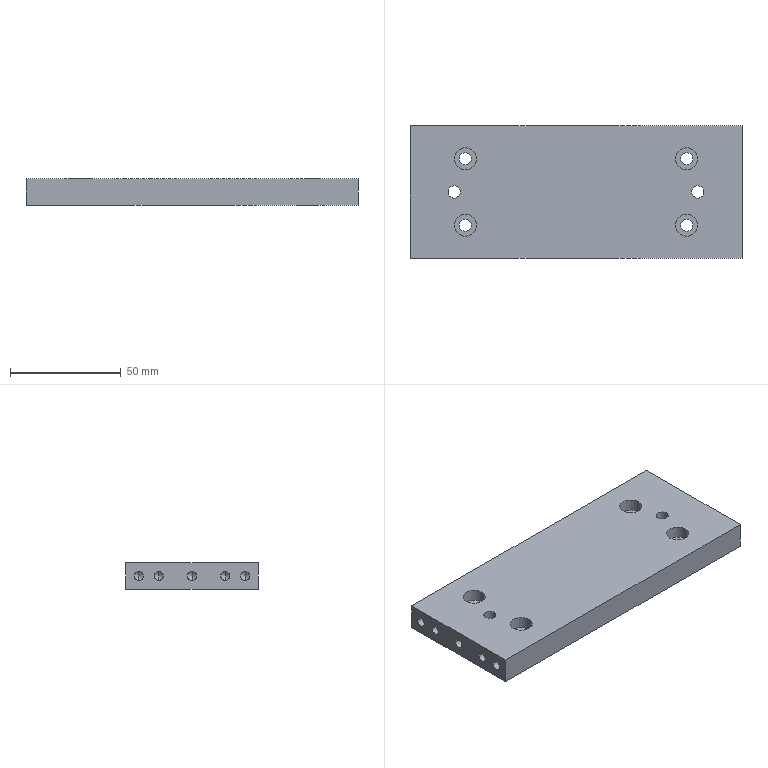Part | SolidWorks | features BaseBody 1 | 1 solid | 76 faces | box 150 x 60 x 12 mm | volume 103321 mm3 | cylinder 44 | cone 20 | plane 12 | commonest cylinder face diameters 4.134 x12 5.5 x12 10 x12 4 x8